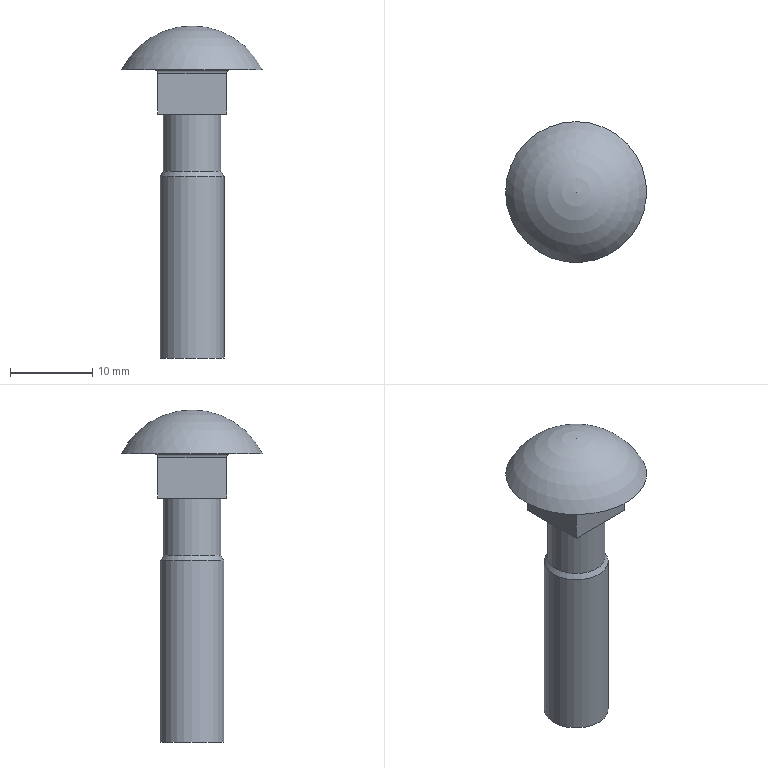Part | NX | features DATUM_CSYS 2, SKETCH 2, BLEND 1, EXTRUDE 1, LINE 1, META 1, SWP104 1, SYMBOLIC_THREAD 1, THREADS 1 | 1 solid | 15 faces | box 17.1 x 17.1 x 40.28 mm | volume 2398 mm3 | plane 7 | cylinder 6 | cone 1 | sphere 1 | commonest cylinder face diameters 1 x4 6.995 x1 7.76 x1
STEP:
#1=CARTESIAN_POINT('',(-3.497,0.,-12.337));
#2=VERTEX_POINT('',#1);
#3=CARTESIAN_POINT('',(0.,0.,-12.337));
#4=DIRECTION('',(0.,0.,-1.));
#5=DIRECTION('',(-1.,0.,0.));
#6=AXIS2_PLACEMENT_3D('',#3,#4,#5);
#7=CIRCLE('',#6,3.497);
#8=EDGE_CURVE('',#2,#2,#7,.T.);
#9=ORIENTED_EDGE('',*,*,#8,.F.);
#10=EDGE_LOOP('',(#9));
#11=FACE_BOUND('',#10,.T.);
#12=CARTESIAN_POINT('',(3.497,0.,-5.4));
#13=VERTEX_POINT('',#12);
#14=CARTESIAN_POINT('',(0.,0.,-5.4));
#15=DIRECTION('',(0.,0.,1.));
#16=DIRECTION('',(1.,0.,0.));
#17=AXIS2_PLACEMENT_3D('',#14,#15,#16);
#18=CIRCLE('',#17,3.497);
#19=EDGE_CURVE('',#13,#13,#18,.F.);
#20=ORIENTED_EDGE('',*,*,#19,.T.);
#21=EDGE_LOOP('',(#20));
#22=FACE_BOUND('',#21,.T.);
#23=CARTESIAN_POINT('',(0.,0.,0.));
#24=DIRECTION('',(0.,0.,-1.));
#25=DIRECTION('',(-1.,0.,0.));
#26=AXIS2_PLACEMENT_3D('',#23,#24,#25);
#27=CYLINDRICAL_SURFACE('',#26,3.497);
#28=ADVANCED_FACE('',(#11,#22),#27,.T.);
#29=ORIENTED_EDGE('',*,*,#8,.T.);
#30=EDGE_LOOP('',(#29));
#31=FACE_BOUND('',#30,.T.);
#32=CARTESIAN_POINT('',(-3.88,0.,-13.));
#33=VERTEX_POINT('',#32);
#34=CARTESIAN_POINT('',(0.,0.,-13.));
#35=DIRECTION('',(0.,0.,-1.));
#36=DIRECTION('',(-1.,0.,0.));
#37=AXIS2_PLACEMENT_3D('',#34,#35,#36);
#38=CIRCLE('',#37,3.88);
#39=EDGE_CURVE('',#33,#33,#38,.T.);
#40=ORIENTED_EDGE('',*,*,#39,.F.);
#41=EDGE_LOOP('',(#40));
#42=FACE_BOUND('',#41,.T.);
#43=CARTESIAN_POINT('',(0.,0.,-13.));
#44=DIRECTION('',(0.,0.,-1.));
#45=DIRECTION('',(-1.,0.,0.));
#46=AXIS2_PLACEMENT_3D('',#43,#44,#45);
#47=CONICAL_SURFACE('',#46,3.88,0.5236);
#48=ADVANCED_FACE('',(#31,#42),#47,.T.);
#49=CARTESIAN_POINT('',(-3.88,0.,-35.));
#50=VERTEX_POINT('',#49);
#51=CARTESIAN_POINT('',(0.,0.,-35.));
#52=DIRECTION('',(0.,0.,-1.));
#53=DIRECTION('',(-1.,0.,0.));
#54=AXIS2_PLACEMENT_3D('',#51,#52,#53);
#55=CIRCLE('',#54,3.88);
#56=EDGE_CURVE('',#50,#50,#55,.T.);
#57=ORIENTED_EDGE('',*,*,#56,.T.);
#58=EDGE_LOOP('',(#57));
#59=FACE_BOUND('',#58,.T.);
#60=CARTESIAN_POINT('',(0.,0.,-35.));
#61=DIRECTION('',(0.,0.,-1.));
#62=DIRECTION('',(-1.,0.,0.));
#63=AXIS2_PLACEMENT_3D('',#60,#61,#62);
#64=PLANE('',#63);
#65=ADVANCED_FACE('',(#59),#64,.T.);
#66=ORIENTED_EDGE('',*,*,#39,.T.);
#67=EDGE_LOOP('',(#66));
#68=FACE_BOUND('',#67,.T.);
#69=ORIENTED_EDGE('',*,*,#56,.F.);
#70=EDGE_LOOP('',(#69));
#71=FACE_BOUND('',#70,.T.);
#72=CARTESIAN_POINT('',(0.,0.,0.));
#73=DIRECTION('',(0.,0.,-1.));
#74=DIRECTION('',(-1.,0.,0.));
#75=AXIS2_PLACEMENT_3D('',#72,#73,#74);
#76=CYLINDRICAL_SURFACE('',#75,3.88);
#77=ADVANCED_FACE('',(#68,#71),#76,.T.);
#78=CARTESIAN_POINT('',(-4.18,-4.18,-5.4));
#79=VERTEX_POINT('',#78);
#80=CARTESIAN_POINT('',(-4.18,-4.18,-0.5));
#81=VERTEX_POINT('',#80);
#82=CARTESIAN_POINT('',(-4.18,-4.18,-5.4));
#83=DIRECTION('',(0.,0.,1.));
#84=VECTOR('',#83,1000.);
#85=LINE('',#82,#84);
#86=EDGE_CURVE('',#79,#81,#85,.T.);
#87=ORIENTED_EDGE('',*,*,#86,.T.);
#88=CARTESIAN_POINT('',(-4.18,4.18,-0.5));
#89=VERTEX_POINT('',#88);
#90=CARTESIAN_POINT('',(-4.18,4.18,-0.5));
#91=DIRECTION('',(0.,-1.,0.));
#92=VECTOR('',#91,1000.);
#93=LINE('',#90,#92);
#94=EDGE_CURVE('',#81,#89,#93,.F.);
#95=ORIENTED_EDGE('',*,*,#94,.T.);
#96=CARTESIAN_POINT('',(-4.18,4.18,-5.4));
#97=VERTEX_POINT('',#96);
#98=CARTESIAN_POINT('',(-4.18,4.18,-5.4));
#99=DIRECTION('',(0.,0.,1.));
#100=VECTOR('',#99,1000.);
#101=LINE('',#98,#100);
#102=EDGE_CURVE('',#97,#89,#101,.T.);
#103=ORIENTED_EDGE('',*,*,#102,.F.);
#104=CARTESIAN_POINT('',(-4.18,4.18,-5.4));
#105=DIRECTION('',(0.,-1.,0.));
#106=VECTOR('',#105,1000.);
#107=LINE('',#104,#106);
#108=EDGE_CURVE('',#97,#79,#107,.T.);
#109=ORIENTED_EDGE('',*,*,#108,.T.);
#110=EDGE_LOOP('',(#87,#95,#103,#109));
#111=FACE_BOUND('',#110,.T.);
#112=CARTESIAN_POINT('',(-4.18,4.18,-5.4));
#113=DIRECTION('',(-1.,0.,0.));
#114=DIRECTION('',(0.,0.,1.));
#115=AXIS2_PLACEMENT_3D('',#112,#113,#114);
#116=PLANE('',#115);
#117=ADVANCED_FACE('',(#111),#116,.T.);
#118=CARTESIAN_POINT('',(4.18,-4.18,-5.4));
#119=VERTEX_POINT('',#118);
#120=CARTESIAN_POINT('',(4.18,-4.18,-0.5));
#121=VERTEX_POINT('',#120);
#122=CARTESIAN_POINT('',(4.18,-4.18,-5.4));
#123=DIRECTION('',(0.,0.,1.));
#124=VECTOR('',#123,1000.);
#125=LINE('',#122,#124);
#126=EDGE_CURVE('',#119,#121,#125,.T.);
#127=ORIENTED_EDGE('',*,*,#126,.T.);
#128=CARTESIAN_POINT('',(-4.18,-4.18,-0.5));
#129=DIRECTION('',(1.,0.,0.));
#130=VECTOR('',#129,1000.);
#131=LINE('',#128,#130);
#132=EDGE_CURVE('',#121,#81,#131,.F.);
#133=ORIENTED_EDGE('',*,*,#132,.T.);
#134=ORIENTED_EDGE('',*,*,#86,.F.);
#135=CARTESIAN_POINT('',(-4.18,-4.18,-5.4));
#136=DIRECTION('',(1.,0.,0.));
#137=VECTOR('',#136,1000.);
#138=LINE('',#135,#137);
#139=EDGE_CURVE('',#79,#119,#138,.T.);
#140=ORIENTED_EDGE('',*,*,#139,.T.);
#141=EDGE_LOOP('',(#127,#133,#134,#140));
#142=FACE_BOUND('',#141,.T.);
#143=CARTESIAN_POINT('',(-4.18,-4.18,-5.4));
#144=DIRECTION('',(0.,-1.,0.));
#145=DIRECTION('',(0.,0.,-1.));
#146=AXIS2_PLACEMENT_3D('',#143,#144,#145);
#147=PLANE('',#146);
#148=ADVANCED_FACE('',(#142),#147,.T.);
#149=CARTESIAN_POINT('',(4.18,4.18,-5.4));
#150=VERTEX_POINT('',#149);
#151=CARTESIAN_POINT('',(4.18,4.18,-0.5));
#152=VERTEX_POINT('',#151);
#153=CARTESIAN_POINT('',(4.18,4.18,-5.4));
#154=DIRECTION('',(0.,0.,1.));
#155=VECTOR('',#154,1000.);
#156=LINE('',#153,#155);
#157=EDGE_CURVE('',#150,#152,#156,.T.);
#158=ORIENTED_EDGE('',*,*,#157,.T.);
#159=CARTESIAN_POINT('',(4.18,-4.18,-0.5));
#160=DIRECTION('',(0.,1.,0.));
#161=VECTOR('',#160,1000.);
#162=LINE('',#159,#161);
#163=EDGE_CURVE('',#152,#121,#162,.F.);
#164=ORIENTED_EDGE('',*,*,#163,.T.);
#165=ORIENTED_EDGE('',*,*,#126,.F.);
#166=CARTESIAN_POINT('',(4.18,-4.18,-5.4));
#167=DIRECTION('',(0.,1.,0.));
#168=VECTOR('',#167,1000.);
#169=LINE('',#166,#168);
#170=EDGE_CURVE('',#119,#150,#169,.T.);
#171=ORIENTED_EDGE('',*,*,#170,.T.);
#172=EDGE_LOOP('',(#158,#164,#165,#171));
#173=FACE_BOUND('',#172,.T.);
#174=CARTESIAN_POINT('',(4.18,-4.18,-5.4));
#175=DIRECTION('',(1.,0.,0.));
#176=DIRECTION('',(0.,0.,-1.));
#177=AXIS2_PLACEMENT_3D('',#174,#175,#176);
#178=PLANE('',#177);
#179=ADVANCED_FACE('',(#173),#178,.T.);
#180=ORIENTED_EDGE('',*,*,#102,.T.);
#181=CARTESIAN_POINT('',(4.18,4.18,-0.5));
#182=DIRECTION('',(-1.,0.,0.));
#183=VECTOR('',#182,1000.);
#184=LINE('',#181,#183);
#185=EDGE_CURVE('',#89,#152,#184,.F.);
#186=ORIENTED_EDGE('',*,*,#185,.T.);
#187=ORIENTED_EDGE('',*,*,#157,.F.);
#188=CARTESIAN_POINT('',(4.18,4.18,-5.4));
#189=DIRECTION('',(-1.,0.,0.));
#190=VECTOR('',#189,1000.);
#191=LINE('',#188,#190);
#192=EDGE_CURVE('',#150,#97,#191,.T.);
#193=ORIENTED_EDGE('',*,*,#192,.T.);
#194=EDGE_LOOP('',(#180,#186,#187,#193));
#195=FACE_BOUND('',#194,.T.);
#196=CARTESIAN_POINT('',(4.18,4.18,-5.4));
#197=DIRECTION('',(0.,1.,0.));
#198=DIRECTION('',(0.,0.,1.));
#199=AXIS2_PLACEMENT_3D('',#196,#197,#198);
#200=PLANE('',#199);
#201=ADVANCED_FACE('',(#195),#200,.T.);
#202=ORIENTED_EDGE('',*,*,#19,.F.);
#203=EDGE_LOOP('',(#202));
#204=FACE_BOUND('',#203,.T.);
#205=ORIENTED_EDGE('',*,*,#108,.F.);
#206=ORIENTED_EDGE('',*,*,#192,.F.);
#207=ORIENTED_EDGE('',*,*,#170,.F.);
#208=ORIENTED_EDGE('',*,*,#139,.F.);
#209=EDGE_LOOP('',(#205,#206,#207,#208));
#210=FACE_BOUND('',#209,.T.);
#211=CARTESIAN_POINT('',(-4.18,-4.18,-5.4));
#212=DIRECTION('',(0.,0.,1.));
#213=DIRECTION('',(1.,0.,0.));
#214=AXIS2_PLACEMENT_3D('',#211,#212,#213);
#215=PLANE('',#214);
#216=ADVANCED_FACE('',(#204,#210),#215,.F.);
#217=CARTESIAN_POINT('',(-8.55,0.,0.));
#218=VERTEX_POINT('',#217);
#219=CARTESIAN_POINT('',(0.,0.,0.));
#220=DIRECTION('',(0.,0.,-1.));
#221=DIRECTION('',(-1.,0.,0.));
#222=AXIS2_PLACEMENT_3D('',#219,#220,#221);
#223=CIRCLE('',#222,8.55);
#224=EDGE_CURVE('',#218,#218,#223,.T.);
#225=ORIENTED_EDGE('',*,*,#224,.F.);
#226=EDGE_LOOP('',(#225));
#227=FACE_BOUND('',#226,.T.);
#228=CARTESIAN_POINT('',(0.,0.,-4.283));
#229=DIRECTION('',(0.,0.,-1.));
#230=DIRECTION('',(0.,1.,0.));
#231=AXIS2_PLACEMENT_3D('',#228,#229,#230);
#232=SPHERICAL_SURFACE('',#231,9.563);
#233=ADVANCED_FACE('',(#227),#232,.T.);
#234=CARTESIAN_POINT('',(-4.68,4.68,0.));
#235=VERTEX_POINT('',#234);
#236=CARTESIAN_POINT('',(-4.68,-4.68,0.));
#237=VERTEX_POINT('',#236);
#238=CARTESIAN_POINT('',(-4.68,-4.18,0.));
#239=DIRECTION('',(0.,-1.,0.));
#240=VECTOR('',#239,1000.);
#241=LINE('',#238,#240);
#242=EDGE_CURVE('',#235,#237,#241,.T.);
#243=ORIENTED_EDGE('',*,*,#242,.T.);
#244=CARTESIAN_POINT('',(4.68,-4.68,0.));
#245=VERTEX_POINT('',#244);
#246=CARTESIAN_POINT('',(4.18,-4.68,0.));
#247=DIRECTION('',(1.,0.,0.));
#248=VECTOR('',#247,1000.);
#249=LINE('',#246,#248);
#250=EDGE_CURVE('',#237,#245,#249,.T.);
#251=ORIENTED_EDGE('',*,*,#250,.T.);
#252=CARTESIAN_POINT('',(4.68,4.68,0.));
#253=VERTEX_POINT('',#252);
#254=CARTESIAN_POINT('',(4.68,4.18,0.));
#255=DIRECTION('',(0.,1.,0.));
#256=VECTOR('',#255,1000.);
#257=LINE('',#254,#256);
#258=EDGE_CURVE('',#245,#253,#257,.T.);
#259=ORIENTED_EDGE('',*,*,#258,.T.);
#260=CARTESIAN_POINT('',(-4.18,4.68,0.));
#261=DIRECTION('',(-1.,0.,0.));
#262=VECTOR('',#261,1000.);
#263=LINE('',#260,#262);
#264=EDGE_CURVE('',#253,#235,#263,.T.);
#265=ORIENTED_EDGE('',*,*,#264,.T.);
#266=EDGE_LOOP('',(#243,#251,#259,#265));
#267=FACE_BOUND('',#266,.T.);
#268=ORIENTED_EDGE('',*,*,#224,.T.);
#269=EDGE_LOOP('',(#268));
#270=FACE_BOUND('',#269,.T.);
#271=CARTESIAN_POINT('',(0.,3.497,0.));
#272=DIRECTION('',(0.,0.,-1.));
#273=DIRECTION('',(-1.,0.,0.));
#274=AXIS2_PLACEMENT_3D('',#271,#272,#273);
#275=PLANE('',#274);
#276=ADVANCED_FACE('',(#267,#270),#275,.T.);
#277=CARTESIAN_POINT('',(4.68,4.68,-0.5));
#278=DIRECTION('',(0.7071,-0.7071,0.));
#279=DIRECTION('',(0.7071,0.7071,0.));
#280=AXIS2_PLACEMENT_3D('',#277,#278,#279);
#281=ELLIPSE('',#280,0.7071,0.5);
#282=EDGE_CURVE('',#152,#253,#281,.F.);
#283=ORIENTED_EDGE('',*,*,#282,.F.);
#284=ORIENTED_EDGE('',*,*,#185,.F.);
#285=CARTESIAN_POINT('',(-4.68,4.68,-0.5));
#286=DIRECTION('',(0.7071,0.7071,0.));
#287=DIRECTION('',(0.7071,-0.7071,0.));
#288=AXIS2_PLACEMENT_3D('',#285,#286,#287);
#289=ELLIPSE('',#288,0.7071,0.5);
#290=EDGE_CURVE('',#235,#89,#289,.T.);
#291=ORIENTED_EDGE('',*,*,#290,.F.);
#292=ORIENTED_EDGE('',*,*,#264,.F.);
#293=EDGE_LOOP('',(#283,#284,#291,#292));
#294=FACE_BOUND('',#293,.T.);
#295=CARTESIAN_POINT('',(0.,4.68,-0.5));
#296=DIRECTION('',(1.,0.,0.));
#297=DIRECTION('',(0.,0.,-1.));
#298=AXIS2_PLACEMENT_3D('',#295,#296,#297);
#299=CYLINDRICAL_SURFACE('',#298,0.5);
#300=ADVANCED_FACE('',(#294),#299,.F.);
#301=ORIENTED_EDGE('',*,*,#290,.T.);
#302=ORIENTED_EDGE('',*,*,#94,.F.);
#303=CARTESIAN_POINT('',(-4.68,-4.68,-0.5));
#304=DIRECTION('',(-0.7071,0.7071,0.));
#305=DIRECTION('',(0.7071,0.7071,0.));
#306=AXIS2_PLACEMENT_3D('',#303,#304,#305);
#307=ELLIPSE('',#306,0.7071,0.5);
#308=EDGE_CURVE('',#237,#81,#307,.T.);
#309=ORIENTED_EDGE('',*,*,#308,.F.);
#310=ORIENTED_EDGE('',*,*,#242,.F.);
#311=EDGE_LOOP('',(#301,#302,#309,#310));
#312=FACE_BOUND('',#311,.T.);
#313=CARTESIAN_POINT('',(-4.68,3.497,-0.5));
#314=DIRECTION('',(0.,1.,0.));
#315=DIRECTION('',(0.,0.,1.));
#316=AXIS2_PLACEMENT_3D('',#313,#314,#315);
#317=CYLINDRICAL_SURFACE('',#316,0.5);
#318=ADVANCED_FACE('',(#312),#317,.F.);
#319=ORIENTED_EDGE('',*,*,#282,.T.);
#320=ORIENTED_EDGE('',*,*,#258,.F.);
#321=CARTESIAN_POINT('',(4.68,-4.68,-0.5));
#322=DIRECTION('',(-0.7071,-0.7071,0.));
#323=DIRECTION('',(0.7071,-0.7071,0.));
#324=AXIS2_PLACEMENT_3D('',#321,#322,#323);
#325=ELLIPSE('',#324,0.7071,0.5);
#326=EDGE_CURVE('',#121,#245,#325,.F.);
#327=ORIENTED_EDGE('',*,*,#326,.F.);
#328=ORIENTED_EDGE('',*,*,#163,.F.);
#329=EDGE_LOOP('',(#319,#320,#327,#328));
#330=FACE_BOUND('',#329,.T.);
#331=CARTESIAN_POINT('',(4.68,3.497,-0.5));
#332=DIRECTION('',(0.,-1.,0.));
#333=DIRECTION('',(0.,0.,-1.));
#334=AXIS2_PLACEMENT_3D('',#331,#332,#333);
#335=CYLINDRICAL_SURFACE('',#334,0.5);
#336=ADVANCED_FACE('',(#330),#335,.F.);
#337=ORIENTED_EDGE('',*,*,#308,.T.);
#338=ORIENTED_EDGE('',*,*,#132,.F.);
#339=ORIENTED_EDGE('',*,*,#326,.T.);
#340=ORIENTED_EDGE('',*,*,#250,.F.);
#341=EDGE_LOOP('',(#337,#338,#339,#340));
#342=FACE_BOUND('',#341,.T.);
#343=CARTESIAN_POINT('',(0.,-4.68,-0.5));
#344=DIRECTION('',(-1.,0.,0.));
#345=DIRECTION('',(0.,0.,1.));
#346=AXIS2_PLACEMENT_3D('',#343,#344,#345);
#347=CYLINDRICAL_SURFACE('',#346,0.5);
#348=ADVANCED_FACE('',(#342),#347,.F.);
#349=CLOSED_SHELL('',(#28,#48,#65,#77,#117,#148,#179,#201,#216,#233,#276,#300,#318,#336,#348));
#350=MANIFOLD_SOLID_BREP('',#349);
#351=(LENGTH_UNIT()NAMED_UNIT(*)SI_UNIT(.MILLI.,.METRE.));
#352=UNCERTAINTY_MEASURE_WITH_UNIT(LENGTH_MEASURE(0.00001),#351,'','');
#353=(NAMED_UNIT(*)PLANE_ANGLE_UNIT()SI_UNIT($,.RADIAN.));
#354=(NAMED_UNIT(*)SI_UNIT($,.STERADIAN.)SOLID_ANGLE_UNIT());
#355=(GEOMETRIC_REPRESENTATION_CONTEXT(3)GLOBAL_UNCERTAINTY_ASSIGNED_CONTEXT((#352))GLOBAL_UNIT_ASSIGNED_CONTEXT((#351,#353,#354))REPRESENTATION_CONTEXT('',''));
#356=ADVANCED_BREP_SHAPE_REPRESENTATION('',(#350),#355);